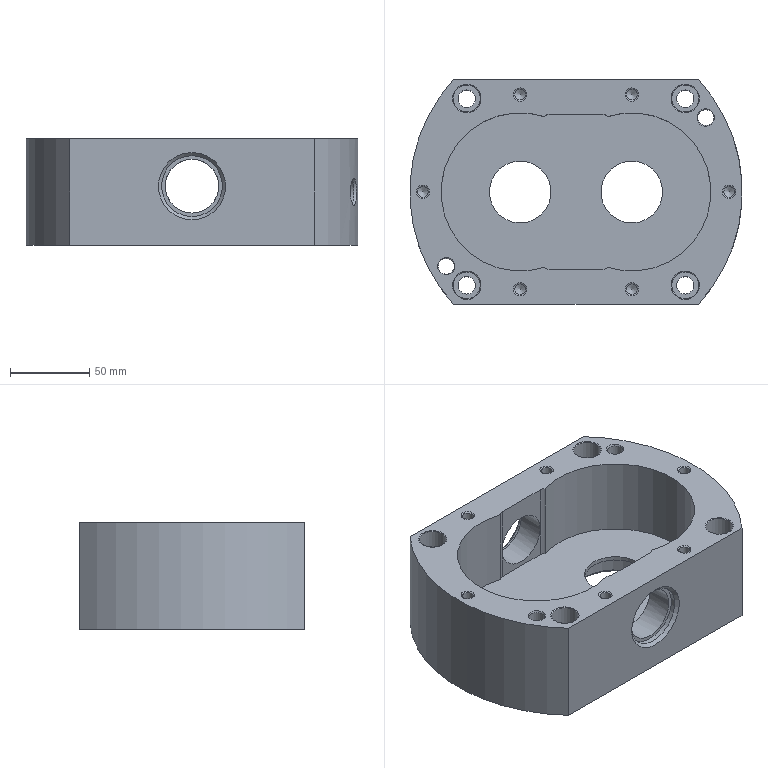NC program | NX | posted with a generic post | part box 210 x 142 x 67.4 mm
Lines 9751 to 10538 of 22889:
(ZLEVEL_PROFILE_COPY_COPY_1 , TOOL : D8)
N19476 T08 M6
N19478 G54
N19480 G17 G0 G90 X-16.947 Y-42.923 B0. C0. S3740 M3
N19482 G43 Z30. H8
N19484 Z-0.1
N19486 G94 G1 X-17.165 Y-44.351 F1000.
N19488 G3 X-16.975 Y-45. R0.8
N19490 G1 X-14.37 F1600.
N19492 G3 X-13.757 Y-44.714 R0.8
N19494 G1 X-12.654 Y-43.4
N19496 G0 X-16.947 Y-42.923 Z-0.2
N19498 G1 X-17.165 Y-44.351 F1000.
N19500 G3 X-16.975 Y-45. R0.8
N19502 G1 X-14.37 F1600.
N19504 G3 X-13.757 Y-44.714 R0.8
N19506 G1 X-12.654 Y-43.4
N19508 G0 X-16.947 Y-42.923 Z-0.3
N19510 G1 X-17.165 Y-44.351 F1000.
N19512 G3 X-16.975 Y-45. R0.8
N19514 G1 X-14.37 F1600.
N19516 G3 X-13.757 Y-44.714 R0.8
N19518 G1 X-12.654 Y-43.4
N19520 G0 X-16.947 Y-42.923 Z-0.4
N19522 G1 X-17.165 Y-44.351 F1000.
N19524 G3 X-16.975 Y-45. R0.8
N19526 G1 X-14.37 F1600.
N19528 G3 X-13.757 Y-44.714 R0.8
N19530 G1 X-12.654 Y-43.4
N19532 G0 X-16.947 Y-42.923 Z-0.5
N19534 G1 X-17.165 Y-44.351 F1000.
N19536 G3 X-16.975 Y-45. R0.8
N19538 G1 X-14.37 F1600.
N19540 G3 X-13.757 Y-44.714 R0.8
N19542 G1 X-12.654 Y-43.4
N19544 G0 X-16.947 Y-42.923 Z-0.6
N19546 G1 X-17.165 Y-44.351 F1000.
N19548 G3 X-16.975 Y-45. R0.8
N19550 G1 X-14.37 F1600.
N19552 G3 X-13.757 Y-44.714 R0.8
N19554 G1 X-12.654 Y-43.4
N19556 G0 X-16.947 Y-42.923 Z-0.7
N19558 G1 X-17.165 Y-44.351 F1000.
N19560 G3 X-16.975 Y-45. R0.8
N19562 G1 X-14.37 F1600.
N19564 G3 X-13.757 Y-44.714 R0.8
N19566 G1 X-12.654 Y-43.4
N19568 G0 X-16.947 Y-42.923 Z-0.8
N19570 G1 X-17.165 Y-44.351 F1000.
N19572 G3 X-16.975 Y-45. R0.8
N19574 G1 X-14.37 F1600.
N19576 G3 X-13.757 Y-44.714 R0.8
N19578 G1 X-12.654 Y-43.4
N19580 G0 X-16.947 Y-42.923 Z-0.9
N19582 G1 X-17.165 Y-44.351 F1000.
N19584 G3 X-16.975 Y-45. R0.8
N19586 G1 X-14.37 F1600.
N19588 G3 X-13.757 Y-44.714 R0.8
N19590 G1 X-12.654 Y-43.4
N19592 G0 X-16.947 Y-42.923 Z-1.
N19594 G1 X-17.165 Y-44.351 F1000.
N19596 G3 X-16.975 Y-45. R0.8
N19598 G1 X-14.37 F1600.
N19600 G3 X-13.757 Y-44.714 R0.8
N19602 G1 X-12.654 Y-43.4
N19604 G0 X-16.947 Y-42.923 Z-1.1
N19606 G1 X-17.165 Y-44.351 F1000.
N19608 G3 X-16.975 Y-45. R0.8
N19610 G1 X-14.37 F1600.
N19612 G3 X-13.757 Y-44.714 R0.8
N19614 G1 X-12.654 Y-43.4
N19616 G0 X-16.947 Y-42.923 Z-1.2
N19618 G1 X-17.165 Y-44.351 F1000.
N19620 G3 X-16.975 Y-45. R0.8
N19622 G1 X-14.37 F1600.
N19624 G3 X-13.757 Y-44.714 R0.8
N19626 G1 X-12.654 Y-43.4
N19628 G0 X-16.947 Y-42.923 Z-1.3
N19630 G1 X-17.165 Y-44.351 F1000.
N19632 G3 X-16.975 Y-45. R0.8
N19634 G1 X-14.37 F1600.
N19636 G3 X-13.757 Y-44.714 R0.8
N19638 G1 X-12.654 Y-43.4
N19640 G0 X-16.947 Y-42.923 Z-1.4
N19642 G1 X-17.165 Y-44.351 F1000.
N19644 G3 X-16.975 Y-45. R0.8
N19646 G1 X-14.37 F1600.
N19648 G3 X-13.757 Y-44.714 R0.8
N19650 G1 X-12.654 Y-43.4
N19652 G0 X-16.947 Y-42.923 Z-1.5
N19654 G1 X-17.165 Y-44.351 F1000.
N19656 G3 X-16.975 Y-45. R0.8
N19658 G1 X-14.37 F1600.
N19660 G3 X-13.757 Y-44.714 R0.8
N19662 G1 X-12.654 Y-43.4
N19664 G0 X-16.947 Y-42.923 Z-1.6
N19666 G1 X-17.165 Y-44.351 F1000.
N19668 G3 X-16.975 Y-45. R0.8
N19670 G1 X-14.37 F1600.
N19672 G3 X-13.757 Y-44.714 R0.8
N19674 G1 X-12.654 Y-43.4
N19676 G0 X-16.947 Y-42.923 Z-1.7
N19678 G1 X-17.165 Y-44.351 F1000.
N19680 G3 X-16.975 Y-45. R0.8
N19682 G1 X-14.37 F1600.
N19684 G3 X-13.757 Y-44.714 R0.8
N19686 G1 X-12.654 Y-43.4
N19688 G0 X-16.947 Y-42.923 Z-1.8
N19690 G1 X-17.165 Y-44.351 F1000.
N19692 G3 X-16.975 Y-45. R0.8
N19694 G1 X-14.37 F1600.
N19696 G3 X-13.757 Y-44.714 R0.8
N19698 G1 X-12.654 Y-43.4
N19700 G0 X-16.947 Y-42.923 Z-1.9
N19702 G1 X-17.165 Y-44.351 F1000.
N19704 G3 X-16.975 Y-45. R0.8
N19706 G1 X-14.37 F1600.
N19708 G3 X-13.757 Y-44.714 R0.8
N19710 G1 X-12.654 Y-43.4
N19712 G0 X-16.947 Y-42.923 Z-2.
N19714 G1 X-17.165 Y-44.351 F1000.
N19716 G3 X-16.975 Y-45. R0.8
N19718 G1 X-14.37 F1600.
N19720 G3 X-13.757 Y-44.714 R0.8
N19722 G1 X-12.654 Y-43.4
N19724 G0 X-16.947 Y-42.923 Z-2.1
N19726 G1 X-17.165 Y-44.351 F1000.
N19728 G3 X-16.975 Y-45. R0.8
N19730 G1 X-14.37 F1600.
N19732 G3 X-13.757 Y-44.714 R0.8
N19734 G1 X-12.654 Y-43.4
N19736 G0 X-16.947 Y-42.923 Z-2.2
N19738 G1 X-17.165 Y-44.351 F1000.
N19740 G3 X-16.975 Y-45. R0.8
N19742 G1 X-14.37 F1600.
N19744 G3 X-13.757 Y-44.714 R0.8
N19746 G1 X-12.654 Y-43.4
N19748 G0 X-16.947 Y-42.923 Z-2.3
N19750 G1 X-17.165 Y-44.351 F1000.
N19752 G3 X-16.975 Y-45. R0.8
N19754 G1 X-14.37 F1600.
N19756 G3 X-13.757 Y-44.714 R0.8
N19758 G1 X-12.654 Y-43.4
N19760 G0 X-16.947 Y-42.923 Z-2.4
N19762 G1 X-17.165 Y-44.351 F1000.
N19764 G3 X-16.975 Y-45. R0.8
N19766 G1 X-14.37 F1600.
N19768 G3 X-13.757 Y-44.714 R0.8
N19770 G1 X-12.654 Y-43.4
N19772 G0 X-16.947 Y-42.923 Z-2.5
N19774 G1 X-17.165 Y-44.351 F1000.
N19776 G3 X-16.975 Y-45. R0.8
N19778 G1 X-14.37 F1600.
N19780 G3 X-13.757 Y-44.714 R0.8
N19782 G1 X-12.654 Y-43.4
N19784 G0 X-16.947 Y-42.923 Z-2.6
N19786 G1 X-17.165 Y-44.351 F1000.
N19788 G3 X-16.975 Y-45. R0.8
N19790 G1 X-14.37 F1600.
N19792 G3 X-13.757 Y-44.714 R0.8
N19794 G1 X-12.654 Y-43.4
N19796 G0 X-16.947 Y-42.923 Z-2.7
N19798 G1 X-17.165 Y-44.351 F1000.
N19800 G3 X-16.975 Y-45. R0.8
N19802 G1 X-14.37 F1600.
N19804 G3 X-13.757 Y-44.714 R0.8
N19806 G1 X-12.654 Y-43.4
N19808 G0 X-16.947 Y-42.923 Z-2.8
N19810 G1 X-17.165 Y-44.351 F1000.
N19812 G3 X-16.975 Y-45. R0.8
N19814 G1 X-14.37 F1600.
N19816 G3 X-13.757 Y-44.714 R0.8
N19818 G1 X-12.654 Y-43.4
N19820 G0 X-16.947 Y-42.923 Z-2.9
N19822 G1 X-17.165 Y-44.351 F1000.
N19824 G3 X-16.975 Y-45. R0.8
N19826 G1 X-14.37 F1600.
N19828 G3 X-13.757 Y-44.714 R0.8
N19830 G1 X-12.654 Y-43.4
N19832 G0 X-16.947 Y-42.923 Z-3.
N19834 G1 X-17.165 Y-44.351 F1000.
N19836 G3 X-16.975 Y-45. R0.8
N19838 G1 X-14.37 F1600.
N19840 G3 X-13.757 Y-44.714 R0.8
N19842 G1 X-12.654 Y-43.4
N19844 G0 X-16.947 Y-42.923 Z-3.1
N19846 G1 X-17.165 Y-44.351 F1000.
N19848 G3 X-16.975 Y-45. R0.8
N19850 G1 X-14.37 F1600.
N19852 G3 X-13.757 Y-44.714 R0.8
N19854 G1 X-12.654 Y-43.4
N19856 G0 X-16.947 Y-42.923 Z-3.2
N19858 G1 X-17.165 Y-44.351 F1000.
N19860 G3 X-16.975 Y-45. R0.8
N19862 G1 X-14.37 F1600.
N19864 G3 X-13.757 Y-44.714 R0.8
N19866 G1 X-12.654 Y-43.4
N19868 G0 X-16.947 Y-42.923 Z-3.3
N19870 G1 X-17.165 Y-44.351 F1000.
N19872 G3 X-16.975 Y-45. R0.8
N19874 G1 X-14.37 F1600.
N19876 G3 X-13.757 Y-44.714 R0.8
N19878 G1 X-12.654 Y-43.4
N19880 G0 X-16.947 Y-42.923 Z-3.4
N19882 G1 X-17.165 Y-44.351 F1000.
N19884 G3 X-16.975 Y-45. R0.8
N19886 G1 X-14.37 F1600.
N19888 G3 X-13.757 Y-44.714 R0.8
N19890 G1 X-12.654 Y-43.4
N19892 G0 X-16.947 Y-42.923 Z-3.5
N19894 G1 X-17.165 Y-44.351 F1000.
N19896 G3 X-16.975 Y-45. R0.8
N19898 G1 X-14.37 F1600.
N19900 G3 X-13.757 Y-44.714 R0.8
N19902 G1 X-12.654 Y-43.4
N19904 G0 X-16.947 Y-42.923 Z-3.6
N19906 G1 X-17.165 Y-44.351 F1000.
N19908 G3 X-16.975 Y-45. R0.8
N19910 G1 X-14.37 F1600.
N19912 G3 X-13.757 Y-44.714 R0.8
N19914 G1 X-12.654 Y-43.4
N19916 G0 X-16.947 Y-42.923 Z-3.7
N19918 G1 X-17.165 Y-44.351 F1000.
N19920 G3 X-16.975 Y-45. R0.8
N19922 G1 X-14.37 F1600.
N19924 G3 X-13.757 Y-44.714 R0.8
N19926 G1 X-12.654 Y-43.4
N19928 G0 X-16.947 Y-42.923 Z-3.8
N19930 G1 X-17.165 Y-44.351 F1000.
N19932 G3 X-16.975 Y-45. R0.8
N19934 G1 X-14.37 F1600.
N19936 G3 X-13.757 Y-44.714 R0.8
N19938 G1 X-12.654 Y-43.4
N19940 G0 X-16.947 Y-42.923 Z-3.9
N19942 G1 X-17.165 Y-44.351 F1000.
N19944 G3 X-16.975 Y-45. R0.8
N19946 G1 X-14.37 F1600.
N19948 G3 X-13.757 Y-44.714 R0.8
N19950 G1 X-12.654 Y-43.4
N19952 G0 X-16.947 Y-42.923 Z-4.
N19954 G1 X-17.165 Y-44.351 F1000.
N19956 G3 X-16.975 Y-45. R0.8
N19958 G1 X-14.37 F1600.
N19960 G3 X-13.757 Y-44.714 R0.8
N19962 G1 X-12.654 Y-43.4
N19964 G0 X-16.947 Y-42.923 Z-4.1
N19966 G1 X-17.165 Y-44.351 F1000.
N19968 G3 X-16.975 Y-45. R0.8
N19970 G1 X-14.37 F1600.
N19972 G3 X-13.757 Y-44.714 R0.8
N19974 G1 X-12.654 Y-43.4
N19976 G0 X-16.947 Y-42.923 Z-4.2
N19978 G1 X-17.165 Y-44.351 F1000.
N19980 G3 X-16.975 Y-45. R0.8
N19982 G1 X-14.37 F1600.
N19984 G3 X-13.757 Y-44.714 R0.8
N19986 G1 X-12.654 Y-43.4
N19988 G0 X-16.947 Y-42.923 Z-4.3
N19990 G1 X-17.165 Y-44.351 F1000.
N19992 G3 X-16.975 Y-45. R0.8
N19994 G1 X-14.37 F1600.
N19996 G3 X-13.757 Y-44.714 R0.8
N19998 G1 X-12.654 Y-43.4
N20000 G0 X-16.947 Y-42.923 Z-4.4
N20002 G1 X-17.165 Y-44.351 F1000.
N20004 G3 X-16.975 Y-45. R0.8
N20006 G1 X-14.37 F1600.
N20008 G3 X-13.757 Y-44.714 R0.8
N20010 G1 X-12.654 Y-43.4
N20012 G0 X-16.947 Y-42.923 Z-4.5
N20014 G1 X-17.165 Y-44.351 F1000.
N20016 G3 X-16.975 Y-45. R0.8
N20018 G1 X-14.37 F1600.
N20020 G3 X-13.757 Y-44.714 R0.8
N20022 G1 X-12.654 Y-43.4
N20024 G0 X-16.947 Y-42.923 Z-4.6
N20026 G1 X-17.165 Y-44.351 F1000.
N20028 G3 X-16.975 Y-45. R0.8
N20030 G1 X-14.37 F1600.
N20032 G3 X-13.757 Y-44.714 R0.8
N20034 G1 X-12.654 Y-43.4
N20036 G0 X-16.947 Y-42.923 Z-4.7
N20038 G1 X-17.165 Y-44.351 F1000.
N20040 G3 X-16.975 Y-45. R0.8
N20042 G1 X-14.37 F1600.
N20044 G3 X-13.757 Y-44.714 R0.8
N20046 G1 X-12.654 Y-43.4
N20048 G0 X-16.947 Y-42.923 Z-4.8
N20050 G1 X-17.165 Y-44.351 F1000.
N20052 G3 X-16.975 Y-45. R0.8
N20054 G1 X-14.37 F1600.
N20056 G3 X-13.757 Y-44.714 R0.8
N20058 G1 X-12.654 Y-43.4
N20060 G0 X-16.947 Y-42.923 Z-4.9
N20062 G1 X-17.165 Y-44.351 F1000.
N20064 G3 X-16.975 Y-45. R0.8
N20066 G1 X-14.37 F1600.
N20068 G3 X-13.757 Y-44.714 R0.8
N20070 G1 X-12.654 Y-43.4
N20072 G0 X-16.947 Y-42.923 Z-5.
N20074 G1 X-17.165 Y-44.351 F1000.
N20076 G3 X-16.975 Y-45. R0.8
N20078 G1 X-14.37 F1600.
N20080 G3 X-13.757 Y-44.714 R0.8
N20082 G1 X-12.654 Y-43.4
N20084 G0 X-16.947 Y-42.923 Z-5.1
N20086 G1 X-17.165 Y-44.351 F1000.
N20088 G3 X-16.975 Y-45. R0.8
N20090 G1 X-14.37 F1600.
N20092 G3 X-13.757 Y-44.714 R0.8
N20094 G1 X-12.654 Y-43.4
N20096 G0 X-16.947 Y-42.923 Z-5.2
N20098 G1 X-17.165 Y-44.351 F1000.
N20100 G3 X-16.975 Y-45. R0.8
N20102 G1 X-14.37 F1600.
N20104 G3 X-13.757 Y-44.714 R0.8
N20106 G1 X-12.654 Y-43.4
N20108 G0 X-16.947 Y-42.923 Z-5.3
N20110 G1 X-17.165 Y-44.351 F1000.
N20112 G3 X-16.975 Y-45. R0.8
N20114 G1 X-14.37 F1600.
N20116 G3 X-13.757 Y-44.714 R0.8
N20118 G1 X-12.654 Y-43.4
N20120 G0 X-16.947 Y-42.923 Z-5.4
N20122 G1 X-17.165 Y-44.351 F1000.
N20124 G3 X-16.975 Y-45. R0.8
N20126 G1 X-14.37 F1600.
N20128 G3 X-13.757 Y-44.714 R0.8
N20130 G1 X-12.654 Y-43.4
N20132 G0 X-16.947 Y-42.923 Z-5.5
N20134 G1 X-17.165 Y-44.351 F1000.
N20136 G3 X-16.975 Y-45. R0.8
N20138 G1 X-14.37 F1600.
N20140 G3 X-13.757 Y-44.714 R0.8
N20142 G1 X-12.654 Y-43.4
N20144 G0 X-16.947 Y-42.923 Z-5.6
N20146 G1 X-17.165 Y-44.351 F1000.
N20148 G3 X-16.975 Y-45. R0.8
N20150 G1 X-14.37 F1600.
N20152 G3 X-13.757 Y-44.714 R0.8
N20154 G1 X-12.654 Y-43.4
N20156 G0 X-16.947 Y-42.923 Z-5.7
N20158 G1 X-17.165 Y-44.351 F1000.
N20160 G3 X-16.975 Y-45. R0.8
N20162 G1 X-14.37 F1600.
N20164 G3 X-13.757 Y-44.714 R0.8
N20166 G1 X-12.654 Y-43.4
N20168 G0 X-16.947 Y-42.923 Z-5.8
N20170 G1 X-17.165 Y-44.351 F1000.
N20172 G3 X-16.975 Y-45. R0.8
N20174 G1 X-14.37 F1600.
N20176 G3 X-13.757 Y-44.714 R0.8
N20178 G1 X-12.654 Y-43.4
N20180 G0 X-16.947 Y-42.923 Z-5.9
N20182 G1 X-17.165 Y-44.351 F1000.
N20184 G3 X-16.975 Y-45. R0.8
N20186 G1 X-14.37 F1600.
N20188 G3 X-13.757 Y-44.714 R0.8
N20190 G1 X-12.654 Y-43.4
N20192 G0 X-16.947 Y-42.923 Z-6.
N20194 G1 X-17.165 Y-44.351 F1000.
N20196 G3 X-16.975 Y-45. R0.8
N20198 G1 X-14.37 F1600.
N20200 G3 X-13.757 Y-44.714 R0.8
N20202 G1 X-12.654 Y-43.4
N20204 G0 X-16.947 Y-42.923 Z-6.1
N20206 G1 X-17.165 Y-44.351 F1000.
N20208 G3 X-16.975 Y-45. R0.8
N20210 G1 X-14.37 F1600.
N20212 G3 X-13.757 Y-44.714 R0.8
N20214 G1 X-12.654 Y-43.4
N20216 G0 X-16.947 Y-42.923 Z-6.2
N20218 G1 X-17.165 Y-44.351 F1000.
N20220 G3 X-16.975 Y-45. R0.8
N20222 G1 X-14.37 F1600.
N20224 G3 X-13.757 Y-44.714 R0.8
N20226 G1 X-12.654 Y-43.4
N20228 G0 X-16.947 Y-42.923 Z-6.3
N20230 G1 X-17.165 Y-44.351 F1000.
N20232 G3 X-16.975 Y-45. R0.8
N20234 G1 X-14.37 F1600.
N20236 G3 X-13.757 Y-44.714 R0.8
N20238 G1 X-12.654 Y-43.4
N20240 G0 X-16.947 Y-42.923 Z-6.4
N20242 G1 X-17.165 Y-44.351 F1000.
N20244 G3 X-16.975 Y-45. R0.8
N20246 G1 X-14.37 F1600.
N20248 G3 X-13.757 Y-44.714 R0.8
N20250 G1 X-12.654 Y-43.4
N20252 G0 X-16.947 Y-42.923 Z-6.5
N20254 G1 X-17.165 Y-44.351 F1000.
N20256 G3 X-16.975 Y-45. R0.8
N20258 G1 X-14.37 F1600.
N20260 G3 X-13.757 Y-44.714 R0.8
N20262 G1 X-12.654 Y-43.4
N20264 G0 X-16.947 Y-42.923 Z-6.6
N20266 G1 X-17.165 Y-44.351 F1000.
N20268 G3 X-16.975 Y-45. R0.8
N20270 G1 X-14.37 F1600.
N20272 G3 X-13.757 Y-44.714 R0.8
N20274 G1 X-12.654 Y-43.4
N20276 G0 X-16.947 Y-42.923 Z-6.7
N20278 G1 X-17.165 Y-44.351 F1000.
N20280 G3 X-16.975 Y-45. R0.8
N20282 G1 X-14.37 F1600.
N20284 G3 X-13.757 Y-44.714 R0.8
N20286 G1 X-12.654 Y-43.4
N20288 G0 X-16.947 Y-42.923 Z-6.8
N20290 G1 X-17.165 Y-44.351 F1000.
N20292 G3 X-16.975 Y-45. R0.8
N20294 G1 X-14.37 F1600.
N20296 G3 X-13.757 Y-44.714 R0.8
N20298 G1 X-12.654 Y-43.4
N20300 G0 X-16.947 Y-42.923 Z-6.9
N20302 G1 X-17.165 Y-44.351 F1000.
N20304 G3 X-16.975 Y-45. R0.8
N20306 G1 X-14.37 F1600.
N20308 G3 X-13.757 Y-44.714 R0.8
N20310 G1 X-12.654 Y-43.4
N20312 G0 X-16.947 Y-42.923 Z-7.
N20314 G1 X-17.165 Y-44.351 F1000.
N20316 G3 X-16.975 Y-45. R0.8
N20318 G1 X-14.37 F1600.
N20320 G3 X-13.757 Y-44.714 R0.8
N20322 G1 X-12.654 Y-43.4
N20324 G0 X-16.947 Y-42.923 Z-7.1
N20326 G1 X-17.165 Y-44.351 F1000.
N20328 G3 X-16.975 Y-45. R0.8
N20330 G1 X-14.37 F1600.
N20332 G3 X-13.757 Y-44.714 R0.8
N20334 G1 X-12.654 Y-43.4
N20336 G0 X-16.947 Y-42.923 Z-7.2
N20338 G1 X-17.165 Y-44.351 F1000.
N20340 G3 X-16.975 Y-45. R0.8
N20342 G1 X-14.37 F1600.
N20344 G3 X-13.757 Y-44.714 R0.8
N20346 G1 X-12.654 Y-43.4
N20348 G0 X-16.947 Y-42.923 Z-7.3
N20350 G1 X-17.165 Y-44.351 F1000.
N20352 G3 X-16.975 Y-45. R0.8
N20354 G1 X-14.37 F1600.
N20356 G3 X-13.757 Y-44.714 R0.8
N20358 G1 X-12.654 Y-43.4
N20360 G0 X-16.947 Y-42.923 Z-7.4
N20362 G1 X-17.165 Y-44.351 F1000.
N20364 G3 X-16.975 Y-45. R0.8
N20366 G1 X-14.37 F1600.
N20368 G3 X-13.757 Y-44.714 R0.8
N20370 G1 X-12.654 Y-43.4
N20372 G0 X-16.947 Y-42.923 Z-7.5
N20374 G1 X-17.165 Y-44.351 F1000.
N20376 G3 X-16.975 Y-45. R0.8
N20378 G1 X-14.37 F1600.
N20380 G3 X-13.757 Y-44.714 R0.8
N20382 G1 X-12.654 Y-43.4
N20384 G0 X-16.947 Y-42.923 Z-7.6
N20386 G1 X-17.165 Y-44.351 F1000.
N20388 G3 X-16.975 Y-45. R0.8
N20390 G1 X-14.37 F1600.
N20392 G3 X-13.757 Y-44.714 R0.8
N20394 G1 X-12.654 Y-43.4
N20396 G0 X-16.947 Y-42.923 Z-7.7
N20398 G1 X-17.165 Y-44.351 F1000.
N20400 G3 X-16.975 Y-45. R0.8
N20402 G1 X-14.37 F1600.
N20404 G3 X-13.757 Y-44.714 R0.8
N20406 G1 X-12.654 Y-43.4
N20408 G0 X-16.947 Y-42.923 Z-7.8
N20410 G1 X-17.165 Y-44.351 F1000.
N20412 G3 X-16.975 Y-45. R0.8
N20414 G1 X-14.37 F1600.
N20416 G3 X-13.757 Y-44.714 R0.8
N20418 G1 X-12.654 Y-43.4
N20420 G0 X-16.947 Y-42.923 Z-7.9
N20422 G1 X-17.165 Y-44.351 F1000.
N20424 G3 X-16.975 Y-45. R0.8
N20426 G1 X-14.37 F1600.
N20428 G3 X-13.757 Y-44.714 R0.8
N20430 G1 X-12.654 Y-43.4
N20432 G0 X-16.947 Y-42.923 Z-8.
N20434 G1 X-17.165 Y-44.351 F1000.
N20436 G3 X-16.975 Y-45. R0.8
N20438 G1 X-14.37 F1600.
N20440 G3 X-13.757 Y-44.714 R0.8
N20442 G1 X-12.654 Y-43.4
N20444 G0 X-16.947 Y-42.923 Z-8.1
N20446 G1 X-17.165 Y-44.351 F1000.
N20448 G3 X-16.975 Y-45. R0.8
N20450 G1 X-14.37 F1600.
N20452 G3 X-13.757 Y-44.714 R0.8
N20454 G1 X-12.654 Y-43.4
N20456 G0 X-16.947 Y-42.923 Z-8.2
N20458 G1 X-17.165 Y-44.351 F1000.
N20460 G3 X-16.975 Y-45. R0.8
N20462 G1 X-14.37 F1600.
N20464 G3 X-13.757 Y-44.714 R0.8
N20466 G1 X-12.654 Y-43.4
N20468 G0 X-16.947 Y-42.923 Z-8.3
N20470 G1 X-17.165 Y-44.351 F1000.
N20472 G3 X-16.975 Y-45. R0.8
N20474 G1 X-14.37 F1600.
N20476 G3 X-13.757 Y-44.714 R0.8
N20478 G1 X-12.654 Y-43.4
N20480 G0 X-16.947 Y-42.923 Z-8.4
N20482 G1 X-17.165 Y-44.351 F1000.
N20484 G3 X-16.975 Y-45. R0.8
N20486 G1 X-14.37 F1600.
N20488 G3 X-13.757 Y-44.714 R0.8
N20490 G1 X-12.654 Y-43.4
N20492 G0 X-16.947 Y-42.923 Z-8.5
N20494 G1 X-17.165 Y-44.351 F1000.
N20496 G3 X-16.975 Y-45. R0.8
N20498 G1 X-14.37 F1600.
N20500 G3 X-13.757 Y-44.714 R0.8
N20502 G1 X-12.654 Y-43.4
N20504 G0 X-16.947 Y-42.923 Z-8.6
N20506 G1 X-17.165 Y-44.351 F1000.
N20508 G3 X-16.975 Y-45. R0.8
N20510 G1 X-14.37 F1600.
N20512 G3 X-13.757 Y-44.714 R0.8
N20514 G1 X-12.654 Y-43.4
N20516 G0 X-16.947 Y-42.923 Z-8.7
N20518 G1 X-17.165 Y-44.351 F1000.
N20520 G3 X-16.975 Y-45. R0.8
N20522 G1 X-14.37 F1600.
N20524 G3 X-13.757 Y-44.714 R0.8
N20526 G1 X-12.654 Y-43.4
N20528 G0 X-16.947 Y-42.923 Z-8.8
N20530 G1 X-17.165 Y-44.351 F1000.
N20532 G3 X-16.975 Y-45. R0.8
N20534 G1 X-14.37 F1600.
N20536 G3 X-13.757 Y-44.714 R0.8
N20538 G1 X-12.654 Y-43.4
N20540 G0 X-16.947 Y-42.923 Z-8.9
N20542 G1 X-17.165 Y-44.351 F1000.
N20544 G3 X-16.975 Y-45. R0.8
N20546 G1 X-14.37 F1600.
N20548 G3 X-13.757 Y-44.714 R0.8
N20550 G1 X-12.654 Y-43.4
N20552 G0 X-16.947 Y-42.923 Z-9.
N20554 G1 X-17.165 Y-44.351 F1000.
N20556 G3 X-16.975 Y-45. R0.8
N20558 G1 X-14.37 F1600.
N20560 G3 X-13.757 Y-44.714 R0.8
N20562 G1 X-12.654 Y-43.4
N20564 G0 X-16.947 Y-42.923 Z-9.1
N20566 G1 X-17.165 Y-44.351 F1000.
N20568 G3 X-16.975 Y-45. R0.8
N20570 G1 X-14.37 F1600.
N20572 G3 X-13.757 Y-44.714 R0.8
N20574 G1 X-12.654 Y-43.4
N20576 G0 X-16.947 Y-42.923 Z-9.2
N20578 G1 X-17.165 Y-44.351 F1000.
N20580 G3 X-16.975 Y-45. R0.8
N20582 G1 X-14.37 F1600.
N20584 G3 X-13.757 Y-44.714 R0.8
N20586 G1 X-12.654 Y-43.4
N20588 G0 X-16.947 Y-42.923 Z-9.3
N20590 G1 X-17.165 Y-44.351 F1000.
N20592 G3 X-16.975 Y-45. R0.8
N20594 G1 X-14.37 F1600.
N20596 G3 X-13.757 Y-44.714 R0.8
N20598 G1 X-12.654 Y-43.4
N20600 G0 X-16.947 Y-42.923 Z-9.4
N20602 G1 X-17.165 Y-44.351 F1000.
N20604 G3 X-16.975 Y-45. R0.8
N20606 G1 X-14.37 F1600.
N20608 G3 X-13.757 Y-44.714 R0.8
N20610 G1 X-12.654 Y-43.4
N20612 G0 X-16.947 Y-42.923 Z-9.5
N20614 G1 X-17.165 Y-44.351 F1000.
N20616 G3 X-16.975 Y-45. R0.8
N20618 G1 X-14.37 F1600.
N20620 G3 X-13.757 Y-44.714 R0.8
N20622 G1 X-12.654 Y-43.4
N20624 G0 X-16.947 Y-42.923 Z-9.6
N20626 G1 X-17.165 Y-44.351 F1000.
N20628 G3 X-16.975 Y-45. R0.8
N20630 G1 X-14.37 F1600.
N20632 G3 X-13.757 Y-44.714 R0.8
N20634 G1 X-12.654 Y-43.4
N20636 G0 X-16.947 Y-42.923 Z-9.7
N20638 G1 X-17.165 Y-44.351 F1000.
N20640 G3 X-16.975 Y-45. R0.8
N20642 G1 X-14.37 F1600.
N20644 G3 X-13.757 Y-44.714 R0.8
N20646 G1 X-12.654 Y-43.4
N20648 G0 X-16.947 Y-42.923 Z-9.8
N20650 G1 X-17.165 Y-44.351 F1000.
N20652 G3 X-16.975 Y-45. R0.8
N20654 G1 X-14.37 F1600.
N20656 G3 X-13.757 Y-44.714 R0.8
N20658 G1 X-12.654 Y-43.4
N20660 G0 X-16.947 Y-42.923 Z-9.9
N20662 G1 X-17.165 Y-44.351 F1000.
N20664 G3 X-16.975 Y-45. R0.8
N20666 G1 X-14.37 F1600.
N20668 G3 X-13.757 Y-44.714 R0.8
N20670 G1 X-12.654 Y-43.4
N20672 G0 X-16.947 Y-42.923 Z-10.
N20674 G1 X-17.165 Y-44.351 F1000.
N20676 G3 X-16.975 Y-45. R0.8
N20678 G1 X-14.37 F1600.
N20680 G3 X-13.757 Y-44.714 R0.8
N20682 G1 X-12.654 Y-43.4
N20684 G0 X-16.947 Y-42.923 Z-10.1
N20686 G1 X-17.165 Y-44.351 F1000.
N20688 G3 X-16.975 Y-45. R0.8
N20690 G1 X-14.37 F1600.
N20692 G3 X-13.757 Y-44.714 R0.8
N20694 G1 X-12.654 Y-43.4
N20696 G0 X-16.947 Y-42.923 Z-10.2
N20698 G1 X-17.165 Y-44.351 F1000.
N20700 G3 X-16.975 Y-45. R0.8
N20702 G1 X-14.37 F1600.
N20704 G3 X-13.757 Y-44.714 R0.8
N20706 G1 X-12.654 Y-43.4
N20708 G0 X-16.947 Y-42.923 Z-10.3
N20710 G1 X-17.165 Y-44.351 F1000.
N20712 G3 X-16.975 Y-45. R0.8
N20714 G1 X-14.37 F1600.
N20716 G3 X-13.757 Y-44.714 R0.8
N20718 G1 X-12.654 Y-43.4
N20720 G0 X-16.947 Y-42.923 Z-10.4
N20722 G1 X-17.165 Y-44.351 F1000.
N20724 G3 X-16.975 Y-45. R0.8
N20726 G1 X-14.37 F1600.
N20728 G3 X-13.757 Y-44.714 R0.8
N20730 G1 X-12.654 Y-43.4
N20732 G0 X-16.947 Y-42.923 Z-10.5
N20734 G1 X-17.165 Y-44.351 F1000.
N20736 G3 X-16.975 Y-45. R0.8
N20738 G1 X-14.37 F1600.
N20740 G3 X-13.757 Y-44.714 R0.8
N20742 G1 X-12.654 Y-43.4
N20744 G0 X-16.947 Y-42.923 Z-10.6
N20746 G1 X-17.165 Y-44.351 F1000.
N20748 G3 X-16.975 Y-45. R0.8
N20750 G1 X-14.37 F1600.
N20752 G3 X-13.757 Y-44.714 R0.8
N20754 G1 X-12.654 Y-43.4
N20756 G0 X-16.947 Y-42.923 Z-10.7
N20758 G1 X-17.165 Y-44.351 F1000.
N20760 G3 X-16.975 Y-45. R0.8
N20762 G1 X-14.37 F1600.
N20764 G3 X-13.757 Y-44.714 R0.8
N20766 G1 X-12.654 Y-43.4
N20768 G0 X-16.947 Y-42.923 Z-10.8
N20770 G1 X-17.165 Y-44.351 F1000.
N20772 G3 X-16.975 Y-45. R0.8
N20774 G1 X-14.37 F1600.
N20776 G3 X-13.757 Y-44.714 R0.8
N20778 G1 X-12.654 Y-43.4
N20780 G0 X-16.947 Y-42.923 Z-10.9
N20782 G1 X-17.165 Y-44.351 F1000.
N20784 G3 X-16.975 Y-45. R0.8
N20786 G1 X-14.37 F1600.
N20788 G3 X-13.757 Y-44.714 R0.8
N20790 G1 X-12.654 Y-43.4
N20792 G0 X-16.947 Y-42.923 Z-11.
N20794 G1 X-17.165 Y-44.351 F1000.
N20796 G3 X-16.975 Y-45. R0.8
N20798 G1 X-14.37 F1600.
N20800 G3 X-13.757 Y-44.714 R0.8
N20802 G1 X-12.654 Y-43.4
N20804 G0 X-16.947 Y-42.923 Z-11.1
N20806 G1 X-17.165 Y-44.351 F1000.
N20808 G3 X-16.975 Y-45. R0.8
N20810 G1 X-14.37 F1600.
N20812 G3 X-13.757 Y-44.714 R0.8
N20814 G1 X-12.654 Y-43.4
N20816 G0 X-16.947 Y-42.923 Z-11.2
N20818 G1 X-17.165 Y-44.351 F1000.
N20820 G3 X-16.975 Y-45. R0.8
N20822 G1 X-14.37 F1600.
N20824 G3 X-13.757 Y-44.714 R0.8
N20826 G1 X-12.654 Y-43.4
N20828 G0 X-16.947 Y-42.923 Z-11.3
N20830 G1 X-17.165 Y-44.351 F1000.
N20832 G3 X-16.975 Y-45. R0.8
N20834 G1 X-14.37 F1600.
N20836 G3 X-13.757 Y-44.714 R0.8
N20838 G1 X-12.654 Y-43.4
N20840 G0 X-16.947 Y-42.923 Z-11.4
N20842 G1 X-17.165 Y-44.351 F1000.
N20844 G3 X-16.975 Y-45. R0.8
N20846 G1 X-14.37 F1600.
N20848 G3 X-13.757 Y-44.714 R0.8
N20850 G1 X-12.654 Y-43.4
N20852 G0 X-16.947 Y-42.923 Z-11.5
N20854 G1 X-17.165 Y-44.351 F1000.
N20856 G3 X-16.975 Y-45. R0.8
N20858 G1 X-14.37 F1600.
N20860 G3 X-13.757 Y-44.714 R0.8
N20862 G1 X-12.654 Y-43.4
N20864 G0 X-16.947 Y-42.923 Z-11.6
N20866 G1 X-17.165 Y-44.351 F1000.
N20868 G3 X-16.975 Y-45. R0.8
N20870 G1 X-14.37 F1600.
N20872 G3 X-13.757 Y-44.714 R0.8
N20874 G1 X-12.654 Y-43.4
N20876 G0 X-16.947 Y-42.923 Z-11.7
N20878 G1 X-17.165 Y-44.351 F1000.
N20880 G3 X-16.975 Y-45. R0.8
N20882 G1 X-14.37 F1600.
N20884 G3 X-13.757 Y-44.714 R0.8
N20886 G1 X-12.654 Y-43.4
N20888 G0 X-16.947 Y-42.923 Z-11.8
N20890 G1 X-17.165 Y-44.351 F1000.
N20892 G3 X-16.975 Y-45. R0.8
N20894 G1 X-14.37 F1600.
N20896 G3 X-13.757 Y-44.714 R0.8
N20898 G1 X-12.654 Y-43.4
N20900 G0 X-16.947 Y-42.923 Z-11.9
N20902 G1 X-17.165 Y-44.351 F1000.
N20904 G3 X-16.975 Y-45. R0.8
N20906 G1 X-14.37 F1600.
N20908 G3 X-13.757 Y-44.714 R0.8
N20910 G1 X-12.654 Y-43.4
N20912 G0 X-16.947 Y-42.923 Z-12.
N20914 G1 X-17.165 Y-44.351 F1000.
N20916 G3 X-16.975 Y-45. R0.8
N20918 G1 X-14.37 F1600.
N20920 G3 X-13.757 Y-44.714 R0.8
N20922 G1 X-12.654 Y-43.4
N20924 G0 X-16.947 Y-42.923 Z-12.1
N20926 G1 X-17.165 Y-44.351 F1000.
N20928 G3 X-16.975 Y-45. R0.8
N20930 G1 X-14.37 F1600.
N20932 G3 X-13.757 Y-44.714 R0.8
N20934 G1 X-12.654 Y-43.4
N20936 G0 X-16.947 Y-42.923 Z-12.2
N20938 G1 X-17.165 Y-44.351 F1000.
N20940 G3 X-16.975 Y-45. R0.8
N20942 G1 X-14.37 F1600.
N20944 G3 X-13.757 Y-44.714 R0.8
N20946 G1 X-12.654 Y-43.4
N20948 G0 X-16.947 Y-42.923 Z-12.3
N20950 G1 X-17.165 Y-44.351 F1000.
N20952 G3 X-16.975 Y-45. R0.8
N20954 G1 X-14.37 F1600.
N20956 G3 X-13.757 Y-44.714 R0.8
N20958 G1 X-12.654 Y-43.4
N20960 G0 X-16.947 Y-42.923 Z-12.4
N20962 G1 X-17.165 Y-44.351 F1000.
N20964 G3 X-16.975 Y-45. R0.8
N20966 G1 X-14.37 F1600.
N20968 G3 X-13.757 Y-44.714 R0.8
N20970 G1 X-12.654 Y-43.4
N20972 G0 X-16.947 Y-42.923 Z-12.5
N20974 G1 X-17.165 Y-44.351 F1000.
N20976 G3 X-16.975 Y-45. R0.8
N20978 G1 X-14.37 F1600.
N20980 G3 X-13.757 Y-44.714 R0.8
N20982 G1 X-12.654 Y-43.4
N20984 G0 X-16.947 Y-42.923 Z-12.6
N20986 G1 X-17.165 Y-44.351 F1000.
N20988 G3 X-16.975 Y-45. R0.8
N20990 G1 X-14.37 F1600.
N20992 G3 X-13.757 Y-44.714 R0.8
N20994 G1 X-12.654 Y-43.4
N20996 G0 X-16.947 Y-42.923 Z-12.7
N20998 G1 X-17.165 Y-44.351 F1000.
N21000 G3 X-16.975 Y-45. R0.8
N21002 G1 X-14.37 F1600.
N21004 G3 X-13.757 Y-44.714 R0.8
N21006 G1 X-12.654 Y-43.4
N21008 G0 X-16.947 Y-42.923 Z-12.8
N21010 G1 X-17.165 Y-44.351 F1000.
N21012 G3 X-16.975 Y-45. R0.8
N21014 G1 X-14.37 F1600.
N21016 G3 X-13.757 Y-44.714 R0.8
N21018 G1 X-12.654 Y-43.4
N21020 G0 X-16.947 Y-42.923 Z-12.9
N21022 G1 X-17.165 Y-44.351 F1000.
N21024 G3 X-16.975 Y-45. R0.8
N21026 G1 X-14.37 F1600.
N21028 G3 X-13.757 Y-44.714 R0.8
N21030 G1 X-12.654 Y-43.4
N21032 G0 X-16.947 Y-42.923 Z-13.
N21034 G1 X-17.165 Y-44.351 F1000.
N21036 G3 X-16.975 Y-45. R0.8
N21038 G1 X-14.37 F1600.
N21040 G3 X-13.757 Y-44.714 R0.8
N21042 G1 X-12.654 Y-43.4
N21044 G0 X-16.947 Y-42.923 Z-13.1